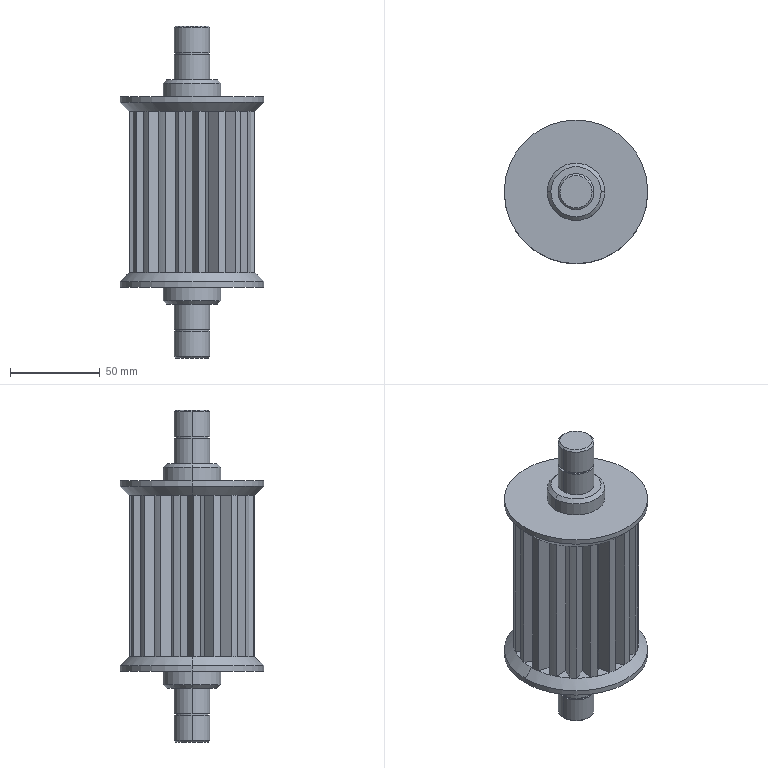Part | STEP file | Floating roller | 1 solid | 137 faces | box 80 x 80 x 185 mm | volume 409392 mm3 | plane 86 | cylinder 39 | cone 12 | commonest cylinder face diameters 70 x19 20 x8 18.5 x4 32 x4 80 x4